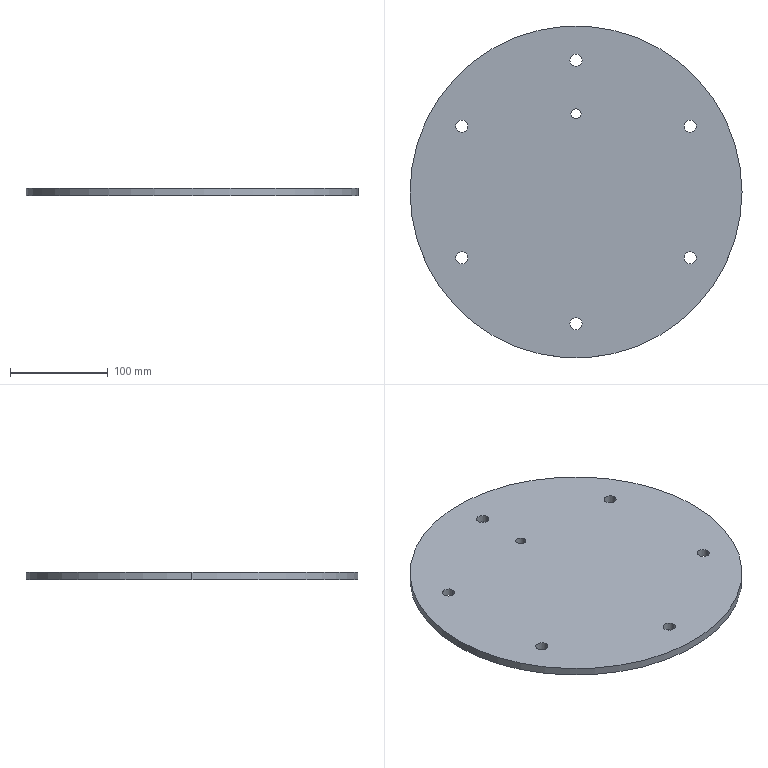Part | SolidWorks | features ICE 2, Extrusion 1 | 1 solid | 18 faces | box 340 x 340 x 8 mm | volume 719786 mm3 | cylinder 16 | plane 2 | commonest cylinder face diameters 12.5 x12 10.25 x2 340 x2
STEP:
#1=CARTESIAN_POINT('',(-5.125,80.,8.));
#2=VERTEX_POINT('',#1);
#3=CARTESIAN_POINT('',(5.125,80.,8.));
#4=VERTEX_POINT('',#3);
#5=CARTESIAN_POINT('',(0.,80.,8.));
#6=DIRECTION('',(0.,0.,1.));
#7=DIRECTION('',(1.,0.,0.));
#8=AXIS2_PLACEMENT_3D('',#5,#6,#7);
#9=CIRCLE('',#8,5.125);
#10=EDGE_CURVE('',#2,#4,#9,.T.);
#11=ORIENTED_EDGE('',*,*,#10,.T.);
#12=CARTESIAN_POINT('',(5.125,80.,0.));
#13=VERTEX_POINT('',#12);
#14=CARTESIAN_POINT('',(5.125,80.,10.));
#15=DIRECTION('',(0.,0.,-1.));
#16=VECTOR('',#15,1000.);
#17=LINE('',#14,#16);
#18=EDGE_CURVE('',#4,#13,#17,.T.);
#19=ORIENTED_EDGE('',*,*,#18,.T.);
#20=CARTESIAN_POINT('',(-5.125,80.,0.));
#21=VERTEX_POINT('',#20);
#22=CARTESIAN_POINT('',(0.,80.,0.));
#23=DIRECTION('',(0.,0.,-1.));
#24=DIRECTION('',(-1.,0.,0.));
#25=AXIS2_PLACEMENT_3D('',#22,#23,#24);
#26=CIRCLE('',#25,5.125);
#27=EDGE_CURVE('',#13,#21,#26,.T.);
#28=ORIENTED_EDGE('',*,*,#27,.T.);
#29=CARTESIAN_POINT('',(-5.125,80.,10.));
#30=DIRECTION('',(0.,0.,-1.));
#31=VECTOR('',#30,1000.);
#32=LINE('',#29,#31);
#33=EDGE_CURVE('',#2,#21,#32,.T.);
#34=ORIENTED_EDGE('',*,*,#33,.F.);
#35=EDGE_LOOP('',(#11,#19,#28,#34));
#36=FACE_OUTER_BOUND('',#35,.T.);
#37=CARTESIAN_POINT('',(0.,80.,10.));
#38=DIRECTION('',(0.,0.,-1.));
#39=DIRECTION('',(-1.,0.,0.));
#40=AXIS2_PLACEMENT_3D('',#37,#38,#39);
#41=CYLINDRICAL_SURFACE('',#40,5.125);
#42=ADVANCED_FACE('',(#36),#41,.F.);
#43=CARTESIAN_POINT('',(110.663,67.5,8.));
#44=VERTEX_POINT('',#43);
#45=CARTESIAN_POINT('',(123.163,67.5,8.));
#46=VERTEX_POINT('',#45);
#47=CARTESIAN_POINT('',(116.913,67.5,8.));
#48=DIRECTION('',(0.,0.,1.));
#49=DIRECTION('',(1.,0.,0.));
#50=AXIS2_PLACEMENT_3D('',#47,#48,#49);
#51=CIRCLE('',#50,6.25);
#52=EDGE_CURVE('',#44,#46,#51,.T.);
#53=ORIENTED_EDGE('',*,*,#52,.T.);
#54=CARTESIAN_POINT('',(123.163,67.5,0.));
#55=VERTEX_POINT('',#54);
#56=CARTESIAN_POINT('',(123.163,67.5,10.));
#57=DIRECTION('',(0.,0.,-1.));
#58=VECTOR('',#57,1000.);
#59=LINE('',#56,#58);
#60=EDGE_CURVE('',#46,#55,#59,.T.);
#61=ORIENTED_EDGE('',*,*,#60,.T.);
#62=CARTESIAN_POINT('',(110.663,67.5,0.));
#63=VERTEX_POINT('',#62);
#64=CARTESIAN_POINT('',(116.913,67.5,0.));
#65=DIRECTION('',(0.,0.,-1.));
#66=DIRECTION('',(-1.,0.,0.));
#67=AXIS2_PLACEMENT_3D('',#64,#65,#66);
#68=CIRCLE('',#67,6.25);
#69=EDGE_CURVE('',#55,#63,#68,.T.);
#70=ORIENTED_EDGE('',*,*,#69,.T.);
#71=CARTESIAN_POINT('',(110.663,67.5,10.));
#72=DIRECTION('',(0.,0.,-1.));
#73=VECTOR('',#72,1000.);
#74=LINE('',#71,#73);
#75=EDGE_CURVE('',#44,#63,#74,.T.);
#76=ORIENTED_EDGE('',*,*,#75,.F.);
#77=EDGE_LOOP('',(#53,#61,#70,#76));
#78=FACE_OUTER_BOUND('',#77,.T.);
#79=CARTESIAN_POINT('',(116.913,67.5,10.));
#80=DIRECTION('',(0.,0.,-1.));
#81=DIRECTION('',(-1.,0.,0.));
#82=AXIS2_PLACEMENT_3D('',#79,#80,#81);
#83=CYLINDRICAL_SURFACE('',#82,6.25);
#84=ADVANCED_FACE('',(#78),#83,.F.);
#85=CARTESIAN_POINT('',(110.663,-67.5,8.));
#86=VERTEX_POINT('',#85);
#87=CARTESIAN_POINT('',(123.163,-67.5,8.));
#88=VERTEX_POINT('',#87);
#89=CARTESIAN_POINT('',(116.913,-67.5,8.));
#90=DIRECTION('',(0.,0.,1.));
#91=DIRECTION('',(1.,0.,0.));
#92=AXIS2_PLACEMENT_3D('',#89,#90,#91);
#93=CIRCLE('',#92,6.25);
#94=EDGE_CURVE('',#86,#88,#93,.T.);
#95=ORIENTED_EDGE('',*,*,#94,.T.);
#96=CARTESIAN_POINT('',(123.163,-67.5,0.));
#97=VERTEX_POINT('',#96);
#98=CARTESIAN_POINT('',(123.163,-67.5,10.));
#99=DIRECTION('',(0.,0.,-1.));
#100=VECTOR('',#99,1000.);
#101=LINE('',#98,#100);
#102=EDGE_CURVE('',#88,#97,#101,.T.);
#103=ORIENTED_EDGE('',*,*,#102,.T.);
#104=CARTESIAN_POINT('',(110.663,-67.5,0.));
#105=VERTEX_POINT('',#104);
#106=CARTESIAN_POINT('',(116.913,-67.5,0.));
#107=DIRECTION('',(0.,0.,-1.));
#108=DIRECTION('',(-1.,0.,0.));
#109=AXIS2_PLACEMENT_3D('',#106,#107,#108);
#110=CIRCLE('',#109,6.25);
#111=EDGE_CURVE('',#97,#105,#110,.T.);
#112=ORIENTED_EDGE('',*,*,#111,.T.);
#113=CARTESIAN_POINT('',(110.663,-67.5,10.));
#114=DIRECTION('',(0.,0.,-1.));
#115=VECTOR('',#114,1000.);
#116=LINE('',#113,#115);
#117=EDGE_CURVE('',#86,#105,#116,.T.);
#118=ORIENTED_EDGE('',*,*,#117,.F.);
#119=EDGE_LOOP('',(#95,#103,#112,#118));
#120=FACE_OUTER_BOUND('',#119,.T.);
#121=CARTESIAN_POINT('',(116.913,-67.5,10.));
#122=DIRECTION('',(0.,0.,-1.));
#123=DIRECTION('',(-1.,0.,0.));
#124=AXIS2_PLACEMENT_3D('',#121,#122,#123);
#125=CYLINDRICAL_SURFACE('',#124,6.25);
#126=ADVANCED_FACE('',(#120),#125,.F.);
#127=CARTESIAN_POINT('',(-6.25,-135.,8.));
#128=VERTEX_POINT('',#127);
#129=CARTESIAN_POINT('',(6.25,-135.,8.));
#130=VERTEX_POINT('',#129);
#131=CARTESIAN_POINT('',(0.,-135.,8.));
#132=DIRECTION('',(0.,0.,1.));
#133=DIRECTION('',(1.,0.,0.));
#134=AXIS2_PLACEMENT_3D('',#131,#132,#133);
#135=CIRCLE('',#134,6.25);
#136=EDGE_CURVE('',#128,#130,#135,.T.);
#137=ORIENTED_EDGE('',*,*,#136,.T.);
#138=CARTESIAN_POINT('',(6.25,-135.,0.));
#139=VERTEX_POINT('',#138);
#140=CARTESIAN_POINT('',(6.25,-135.,10.));
#141=DIRECTION('',(0.,0.,-1.));
#142=VECTOR('',#141,1000.);
#143=LINE('',#140,#142);
#144=EDGE_CURVE('',#130,#139,#143,.T.);
#145=ORIENTED_EDGE('',*,*,#144,.T.);
#146=CARTESIAN_POINT('',(-6.25,-135.,0.));
#147=VERTEX_POINT('',#146);
#148=CARTESIAN_POINT('',(0.,-135.,0.));
#149=DIRECTION('',(0.,0.,-1.));
#150=DIRECTION('',(-1.,0.,0.));
#151=AXIS2_PLACEMENT_3D('',#148,#149,#150);
#152=CIRCLE('',#151,6.25);
#153=EDGE_CURVE('',#139,#147,#152,.T.);
#154=ORIENTED_EDGE('',*,*,#153,.T.);
#155=CARTESIAN_POINT('',(-6.25,-135.,10.));
#156=DIRECTION('',(0.,0.,-1.));
#157=VECTOR('',#156,1000.);
#158=LINE('',#155,#157);
#159=EDGE_CURVE('',#128,#147,#158,.T.);
#160=ORIENTED_EDGE('',*,*,#159,.F.);
#161=EDGE_LOOP('',(#137,#145,#154,#160));
#162=FACE_OUTER_BOUND('',#161,.T.);
#163=CARTESIAN_POINT('',(0.,-135.,10.));
#164=DIRECTION('',(0.,0.,-1.));
#165=DIRECTION('',(-1.,0.,0.));
#166=AXIS2_PLACEMENT_3D('',#163,#164,#165);
#167=CYLINDRICAL_SURFACE('',#166,6.25);
#168=ADVANCED_FACE('',(#162),#167,.F.);
#169=CARTESIAN_POINT('',(-123.163,-67.5,8.));
#170=VERTEX_POINT('',#169);
#171=CARTESIAN_POINT('',(-110.663,-67.5,8.));
#172=VERTEX_POINT('',#171);
#173=CARTESIAN_POINT('',(-116.913,-67.5,8.));
#174=DIRECTION('',(0.,0.,1.));
#175=DIRECTION('',(1.,0.,0.));
#176=AXIS2_PLACEMENT_3D('',#173,#174,#175);
#177=CIRCLE('',#176,6.25);
#178=EDGE_CURVE('',#170,#172,#177,.T.);
#179=ORIENTED_EDGE('',*,*,#178,.T.);
#180=CARTESIAN_POINT('',(-110.663,-67.5,0.));
#181=VERTEX_POINT('',#180);
#182=CARTESIAN_POINT('',(-110.663,-67.5,10.));
#183=DIRECTION('',(0.,0.,-1.));
#184=VECTOR('',#183,1000.);
#185=LINE('',#182,#184);
#186=EDGE_CURVE('',#172,#181,#185,.T.);
#187=ORIENTED_EDGE('',*,*,#186,.T.);
#188=CARTESIAN_POINT('',(-123.163,-67.5,0.));
#189=VERTEX_POINT('',#188);
#190=CARTESIAN_POINT('',(-116.913,-67.5,0.));
#191=DIRECTION('',(0.,0.,-1.));
#192=DIRECTION('',(-1.,0.,0.));
#193=AXIS2_PLACEMENT_3D('',#190,#191,#192);
#194=CIRCLE('',#193,6.25);
#195=EDGE_CURVE('',#181,#189,#194,.T.);
#196=ORIENTED_EDGE('',*,*,#195,.T.);
#197=CARTESIAN_POINT('',(-123.163,-67.5,10.));
#198=DIRECTION('',(0.,0.,-1.));
#199=VECTOR('',#198,1000.);
#200=LINE('',#197,#199);
#201=EDGE_CURVE('',#170,#189,#200,.T.);
#202=ORIENTED_EDGE('',*,*,#201,.F.);
#203=EDGE_LOOP('',(#179,#187,#196,#202));
#204=FACE_OUTER_BOUND('',#203,.T.);
#205=CARTESIAN_POINT('',(-116.913,-67.5,10.));
#206=DIRECTION('',(0.,0.,-1.));
#207=DIRECTION('',(-1.,0.,0.));
#208=AXIS2_PLACEMENT_3D('',#205,#206,#207);
#209=CYLINDRICAL_SURFACE('',#208,6.25);
#210=ADVANCED_FACE('',(#204),#209,.F.);
#211=CARTESIAN_POINT('',(-123.163,67.5,8.));
#212=VERTEX_POINT('',#211);
#213=CARTESIAN_POINT('',(-110.663,67.5,8.));
#214=VERTEX_POINT('',#213);
#215=CARTESIAN_POINT('',(-116.913,67.5,8.));
#216=DIRECTION('',(0.,0.,1.));
#217=DIRECTION('',(1.,0.,0.));
#218=AXIS2_PLACEMENT_3D('',#215,#216,#217);
#219=CIRCLE('',#218,6.25);
#220=EDGE_CURVE('',#212,#214,#219,.T.);
#221=ORIENTED_EDGE('',*,*,#220,.T.);
#222=CARTESIAN_POINT('',(-110.663,67.5,0.));
#223=VERTEX_POINT('',#222);
#224=CARTESIAN_POINT('',(-110.663,67.5,10.));
#225=DIRECTION('',(0.,0.,-1.));
#226=VECTOR('',#225,1000.);
#227=LINE('',#224,#226);
#228=EDGE_CURVE('',#214,#223,#227,.T.);
#229=ORIENTED_EDGE('',*,*,#228,.T.);
#230=CARTESIAN_POINT('',(-123.163,67.5,0.));
#231=VERTEX_POINT('',#230);
#232=CARTESIAN_POINT('',(-116.913,67.5,0.));
#233=DIRECTION('',(0.,0.,-1.));
#234=DIRECTION('',(-1.,0.,0.));
#235=AXIS2_PLACEMENT_3D('',#232,#233,#234);
#236=CIRCLE('',#235,6.25);
#237=EDGE_CURVE('',#223,#231,#236,.T.);
#238=ORIENTED_EDGE('',*,*,#237,.T.);
#239=CARTESIAN_POINT('',(-123.163,67.5,10.));
#240=DIRECTION('',(0.,0.,-1.));
#241=VECTOR('',#240,1000.);
#242=LINE('',#239,#241);
#243=EDGE_CURVE('',#212,#231,#242,.T.);
#244=ORIENTED_EDGE('',*,*,#243,.F.);
#245=EDGE_LOOP('',(#221,#229,#238,#244));
#246=FACE_OUTER_BOUND('',#245,.T.);
#247=CARTESIAN_POINT('',(-116.913,67.5,10.));
#248=DIRECTION('',(0.,0.,-1.));
#249=DIRECTION('',(-1.,0.,0.));
#250=AXIS2_PLACEMENT_3D('',#247,#248,#249);
#251=CYLINDRICAL_SURFACE('',#250,6.25);
#252=ADVANCED_FACE('',(#246),#251,.F.);
#253=CARTESIAN_POINT('',(-6.25,135.,8.));
#254=VERTEX_POINT('',#253);
#255=CARTESIAN_POINT('',(6.25,135.,8.));
#256=VERTEX_POINT('',#255);
#257=CARTESIAN_POINT('',(0.,135.,8.));
#258=DIRECTION('',(0.,0.,1.));
#259=DIRECTION('',(1.,0.,0.));
#260=AXIS2_PLACEMENT_3D('',#257,#258,#259);
#261=CIRCLE('',#260,6.25);
#262=EDGE_CURVE('',#254,#256,#261,.T.);
#263=ORIENTED_EDGE('',*,*,#262,.T.);
#264=CARTESIAN_POINT('',(6.25,135.,0.));
#265=VERTEX_POINT('',#264);
#266=CARTESIAN_POINT('',(6.25,135.,10.));
#267=DIRECTION('',(0.,0.,-1.));
#268=VECTOR('',#267,1000.);
#269=LINE('',#266,#268);
#270=EDGE_CURVE('',#256,#265,#269,.T.);
#271=ORIENTED_EDGE('',*,*,#270,.T.);
#272=CARTESIAN_POINT('',(-6.25,135.,0.));
#273=VERTEX_POINT('',#272);
#274=CARTESIAN_POINT('',(0.,135.,0.));
#275=DIRECTION('',(0.,0.,-1.));
#276=DIRECTION('',(-1.,0.,0.));
#277=AXIS2_PLACEMENT_3D('',#274,#275,#276);
#278=CIRCLE('',#277,6.25);
#279=EDGE_CURVE('',#265,#273,#278,.T.);
#280=ORIENTED_EDGE('',*,*,#279,.T.);
#281=CARTESIAN_POINT('',(-6.25,135.,10.));
#282=DIRECTION('',(0.,0.,-1.));
#283=VECTOR('',#282,1000.);
#284=LINE('',#281,#283);
#285=EDGE_CURVE('',#254,#273,#284,.T.);
#286=ORIENTED_EDGE('',*,*,#285,.F.);
#287=EDGE_LOOP('',(#263,#271,#280,#286));
#288=FACE_OUTER_BOUND('',#287,.T.);
#289=CARTESIAN_POINT('',(0.,135.,10.));
#290=DIRECTION('',(0.,0.,-1.));
#291=DIRECTION('',(-1.,0.,0.));
#292=AXIS2_PLACEMENT_3D('',#289,#290,#291);
#293=CYLINDRICAL_SURFACE('',#292,6.25);
#294=ADVANCED_FACE('',(#288),#293,.F.);
#295=CARTESIAN_POINT('',(170.,0.,8.));
#296=VERTEX_POINT('',#295);
#297=CARTESIAN_POINT('',(-170.,0.,8.));
#298=VERTEX_POINT('',#297);
#299=CARTESIAN_POINT('',(0.,0.,8.));
#300=DIRECTION('',(0.,0.,1.));
#301=DIRECTION('',(1.,0.,0.));
#302=AXIS2_PLACEMENT_3D('',#299,#300,#301);
#303=CIRCLE('',#302,170.);
#304=EDGE_CURVE('',#296,#298,#303,.T.);
#305=ORIENTED_EDGE('',*,*,#304,.F.);
#306=CARTESIAN_POINT('',(170.,0.,0.));
#307=VERTEX_POINT('',#306);
#308=CARTESIAN_POINT('',(170.,0.,8.));
#309=DIRECTION('',(0.,0.,-1.));
#310=VECTOR('',#309,1000.);
#311=LINE('',#308,#310);
#312=EDGE_CURVE('',#296,#307,#311,.T.);
#313=ORIENTED_EDGE('',*,*,#312,.T.);
#314=CARTESIAN_POINT('',(-170.,0.,0.));
#315=VERTEX_POINT('',#314);
#316=CARTESIAN_POINT('',(0.,0.,0.));
#317=DIRECTION('',(0.,0.,1.));
#318=DIRECTION('',(1.,0.,0.));
#319=AXIS2_PLACEMENT_3D('',#316,#317,#318);
#320=CIRCLE('',#319,170.);
#321=EDGE_CURVE('',#307,#315,#320,.T.);
#322=ORIENTED_EDGE('',*,*,#321,.T.);
#323=CARTESIAN_POINT('',(-170.,0.,8.));
#324=DIRECTION('',(0.,0.,-1.));
#325=VECTOR('',#324,1000.);
#326=LINE('',#323,#325);
#327=EDGE_CURVE('',#298,#315,#326,.T.);
#328=ORIENTED_EDGE('',*,*,#327,.F.);
#329=EDGE_LOOP('',(#305,#313,#322,#328));
#330=FACE_OUTER_BOUND('',#329,.T.);
#331=CARTESIAN_POINT('',(0.,0.,8.));
#332=DIRECTION('',(0.,0.,-1.));
#333=DIRECTION('',(-1.,0.,0.));
#334=AXIS2_PLACEMENT_3D('',#331,#332,#333);
#335=CYLINDRICAL_SURFACE('',#334,170.);
#336=ADVANCED_FACE('',(#330),#335,.T.);
#337=ORIENTED_EDGE('',*,*,#312,.F.);
#338=CARTESIAN_POINT('',(0.,0.,8.));
#339=DIRECTION('',(0.,0.,1.));
#340=DIRECTION('',(1.,0.,0.));
#341=AXIS2_PLACEMENT_3D('',#338,#339,#340);
#342=CIRCLE('',#341,170.);
#343=EDGE_CURVE('',#298,#296,#342,.T.);
#344=ORIENTED_EDGE('',*,*,#343,.F.);
#345=ORIENTED_EDGE('',*,*,#327,.T.);
#346=CARTESIAN_POINT('',(0.,0.,0.));
#347=DIRECTION('',(0.,0.,1.));
#348=DIRECTION('',(1.,0.,0.));
#349=AXIS2_PLACEMENT_3D('',#346,#347,#348);
#350=CIRCLE('',#349,170.);
#351=EDGE_CURVE('',#315,#307,#350,.T.);
#352=ORIENTED_EDGE('',*,*,#351,.T.);
#353=EDGE_LOOP('',(#337,#344,#345,#352));
#354=FACE_OUTER_BOUND('',#353,.T.);
#355=CARTESIAN_POINT('',(0.,0.,8.));
#356=DIRECTION('',(0.,0.,-1.));
#357=DIRECTION('',(-1.,0.,0.));
#358=AXIS2_PLACEMENT_3D('',#355,#356,#357);
#359=CYLINDRICAL_SURFACE('',#358,170.);
#360=ADVANCED_FACE('',(#354),#359,.T.);
#361=ORIENTED_EDGE('',*,*,#10,.F.);
#362=CARTESIAN_POINT('',(0.,80.,8.));
#363=DIRECTION('',(0.,0.,1.));
#364=DIRECTION('',(1.,0.,0.));
#365=AXIS2_PLACEMENT_3D('',#362,#363,#364);
#366=CIRCLE('',#365,5.125);
#367=EDGE_CURVE('',#4,#2,#366,.T.);
#368=ORIENTED_EDGE('',*,*,#367,.F.);
#369=EDGE_LOOP('',(#361,#368));
#370=FACE_BOUND('',#369,.T.);
#371=ORIENTED_EDGE('',*,*,#52,.F.);
#372=CARTESIAN_POINT('',(116.913,67.5,8.));
#373=DIRECTION('',(0.,0.,1.));
#374=DIRECTION('',(1.,0.,0.));
#375=AXIS2_PLACEMENT_3D('',#372,#373,#374);
#376=CIRCLE('',#375,6.25);
#377=EDGE_CURVE('',#46,#44,#376,.T.);
#378=ORIENTED_EDGE('',*,*,#377,.F.);
#379=EDGE_LOOP('',(#371,#378));
#380=FACE_BOUND('',#379,.T.);
#381=ORIENTED_EDGE('',*,*,#94,.F.);
#382=CARTESIAN_POINT('',(116.913,-67.5,8.));
#383=DIRECTION('',(0.,0.,1.));
#384=DIRECTION('',(1.,0.,0.));
#385=AXIS2_PLACEMENT_3D('',#382,#383,#384);
#386=CIRCLE('',#385,6.25);
#387=EDGE_CURVE('',#88,#86,#386,.T.);
#388=ORIENTED_EDGE('',*,*,#387,.F.);
#389=EDGE_LOOP('',(#381,#388));
#390=FACE_BOUND('',#389,.T.);
#391=ORIENTED_EDGE('',*,*,#136,.F.);
#392=CARTESIAN_POINT('',(0.,-135.,8.));
#393=DIRECTION('',(0.,0.,1.));
#394=DIRECTION('',(1.,0.,0.));
#395=AXIS2_PLACEMENT_3D('',#392,#393,#394);
#396=CIRCLE('',#395,6.25);
#397=EDGE_CURVE('',#130,#128,#396,.T.);
#398=ORIENTED_EDGE('',*,*,#397,.F.);
#399=EDGE_LOOP('',(#391,#398));
#400=FACE_BOUND('',#399,.T.);
#401=ORIENTED_EDGE('',*,*,#178,.F.);
#402=CARTESIAN_POINT('',(-116.913,-67.5,8.));
#403=DIRECTION('',(0.,0.,1.));
#404=DIRECTION('',(1.,0.,0.));
#405=AXIS2_PLACEMENT_3D('',#402,#403,#404);
#406=CIRCLE('',#405,6.25);
#407=EDGE_CURVE('',#172,#170,#406,.T.);
#408=ORIENTED_EDGE('',*,*,#407,.F.);
#409=EDGE_LOOP('',(#401,#408));
#410=FACE_BOUND('',#409,.T.);
#411=ORIENTED_EDGE('',*,*,#220,.F.);
#412=CARTESIAN_POINT('',(-116.913,67.5,8.));
#413=DIRECTION('',(0.,0.,1.));
#414=DIRECTION('',(1.,0.,0.));
#415=AXIS2_PLACEMENT_3D('',#412,#413,#414);
#416=CIRCLE('',#415,6.25);
#417=EDGE_CURVE('',#214,#212,#416,.T.);
#418=ORIENTED_EDGE('',*,*,#417,.F.);
#419=EDGE_LOOP('',(#411,#418));
#420=FACE_BOUND('',#419,.T.);
#421=ORIENTED_EDGE('',*,*,#262,.F.);
#422=CARTESIAN_POINT('',(0.,135.,8.));
#423=DIRECTION('',(0.,0.,1.));
#424=DIRECTION('',(1.,0.,0.));
#425=AXIS2_PLACEMENT_3D('',#422,#423,#424);
#426=CIRCLE('',#425,6.25);
#427=EDGE_CURVE('',#256,#254,#426,.T.);
#428=ORIENTED_EDGE('',*,*,#427,.F.);
#429=EDGE_LOOP('',(#421,#428));
#430=FACE_BOUND('',#429,.T.);
#431=ORIENTED_EDGE('',*,*,#343,.T.);
#432=ORIENTED_EDGE('',*,*,#304,.T.);
#433=EDGE_LOOP('',(#431,#432));
#434=FACE_OUTER_BOUND('',#433,.T.);
#435=CARTESIAN_POINT('',(0.,0.,8.));
#436=DIRECTION('',(0.,0.,1.));
#437=DIRECTION('',(1.,0.,0.));
#438=AXIS2_PLACEMENT_3D('',#435,#436,#437);
#439=PLANE('',#438);
#440=ADVANCED_FACE('',(#370,#380,#390,#400,#410,#420,#430,#434),#439,.T.);
#441=CARTESIAN_POINT('',(0.,80.,0.));
#442=DIRECTION('',(0.,0.,-1.));
#443=DIRECTION('',(-1.,0.,0.));
#444=AXIS2_PLACEMENT_3D('',#441,#442,#443);
#445=CIRCLE('',#444,5.125);
#446=EDGE_CURVE('',#21,#13,#445,.T.);
#447=ORIENTED_EDGE('',*,*,#446,.F.);
#448=ORIENTED_EDGE('',*,*,#27,.F.);
#449=EDGE_LOOP('',(#447,#448));
#450=FACE_BOUND('',#449,.T.);
#451=CARTESIAN_POINT('',(116.913,67.5,0.));
#452=DIRECTION('',(0.,0.,-1.));
#453=DIRECTION('',(-1.,0.,0.));
#454=AXIS2_PLACEMENT_3D('',#451,#452,#453);
#455=CIRCLE('',#454,6.25);
#456=EDGE_CURVE('',#63,#55,#455,.T.);
#457=ORIENTED_EDGE('',*,*,#456,.F.);
#458=ORIENTED_EDGE('',*,*,#69,.F.);
#459=EDGE_LOOP('',(#457,#458));
#460=FACE_BOUND('',#459,.T.);
#461=CARTESIAN_POINT('',(116.913,-67.5,0.));
#462=DIRECTION('',(0.,0.,-1.));
#463=DIRECTION('',(-1.,0.,0.));
#464=AXIS2_PLACEMENT_3D('',#461,#462,#463);
#465=CIRCLE('',#464,6.25);
#466=EDGE_CURVE('',#105,#97,#465,.T.);
#467=ORIENTED_EDGE('',*,*,#466,.F.);
#468=ORIENTED_EDGE('',*,*,#111,.F.);
#469=EDGE_LOOP('',(#467,#468));
#470=FACE_BOUND('',#469,.T.);
#471=CARTESIAN_POINT('',(0.,-135.,0.));
#472=DIRECTION('',(0.,0.,-1.));
#473=DIRECTION('',(-1.,0.,0.));
#474=AXIS2_PLACEMENT_3D('',#471,#472,#473);
#475=CIRCLE('',#474,6.25);
#476=EDGE_CURVE('',#147,#139,#475,.T.);
#477=ORIENTED_EDGE('',*,*,#476,.F.);
#478=ORIENTED_EDGE('',*,*,#153,.F.);
#479=EDGE_LOOP('',(#477,#478));
#480=FACE_BOUND('',#479,.T.);
#481=CARTESIAN_POINT('',(-116.913,-67.5,0.));
#482=DIRECTION('',(0.,0.,-1.));
#483=DIRECTION('',(-1.,0.,0.));
#484=AXIS2_PLACEMENT_3D('',#481,#482,#483);
#485=CIRCLE('',#484,6.25);
#486=EDGE_CURVE('',#189,#181,#485,.T.);
#487=ORIENTED_EDGE('',*,*,#486,.F.);
#488=ORIENTED_EDGE('',*,*,#195,.F.);
#489=EDGE_LOOP('',(#487,#488));
#490=FACE_BOUND('',#489,.T.);
#491=CARTESIAN_POINT('',(-116.913,67.5,0.));
#492=DIRECTION('',(0.,0.,-1.));
#493=DIRECTION('',(-1.,0.,0.));
#494=AXIS2_PLACEMENT_3D('',#491,#492,#493);
#495=CIRCLE('',#494,6.25);
#496=EDGE_CURVE('',#231,#223,#495,.T.);
#497=ORIENTED_EDGE('',*,*,#496,.F.);
#498=ORIENTED_EDGE('',*,*,#237,.F.);
#499=EDGE_LOOP('',(#497,#498));
#500=FACE_BOUND('',#499,.T.);
#501=CARTESIAN_POINT('',(0.,135.,0.));
#502=DIRECTION('',(0.,0.,-1.));
#503=DIRECTION('',(-1.,0.,0.));
#504=AXIS2_PLACEMENT_3D('',#501,#502,#503);
#505=CIRCLE('',#504,6.25);
#506=EDGE_CURVE('',#273,#265,#505,.T.);
#507=ORIENTED_EDGE('',*,*,#506,.F.);
#508=ORIENTED_EDGE('',*,*,#279,.F.);
#509=EDGE_LOOP('',(#507,#508));
#510=FACE_BOUND('',#509,.T.);
#511=ORIENTED_EDGE('',*,*,#351,.F.);
#512=ORIENTED_EDGE('',*,*,#321,.F.);
#513=EDGE_LOOP('',(#511,#512));
#514=FACE_OUTER_BOUND('',#513,.T.);
#515=CARTESIAN_POINT('',(0.,0.,0.));
#516=DIRECTION('',(0.,0.,1.));
#517=DIRECTION('',(1.,0.,0.));
#518=AXIS2_PLACEMENT_3D('',#515,#516,#517);
#519=PLANE('',#518);
#520=ADVANCED_FACE('',(#450,#460,#470,#480,#490,#500,#510,#514),#519,.F.);
#521=ORIENTED_EDGE('',*,*,#270,.F.);
#522=ORIENTED_EDGE('',*,*,#427,.T.);
#523=ORIENTED_EDGE('',*,*,#285,.T.);
#524=ORIENTED_EDGE('',*,*,#506,.T.);
#525=EDGE_LOOP('',(#521,#522,#523,#524));
#526=FACE_OUTER_BOUND('',#525,.T.);
#527=CARTESIAN_POINT('',(0.,135.,10.));
#528=DIRECTION('',(0.,0.,-1.));
#529=DIRECTION('',(-1.,0.,0.));
#530=AXIS2_PLACEMENT_3D('',#527,#528,#529);
#531=CYLINDRICAL_SURFACE('',#530,6.25);
#532=ADVANCED_FACE('',(#526),#531,.F.);
#533=ORIENTED_EDGE('',*,*,#228,.F.);
#534=ORIENTED_EDGE('',*,*,#417,.T.);
#535=ORIENTED_EDGE('',*,*,#243,.T.);
#536=ORIENTED_EDGE('',*,*,#496,.T.);
#537=EDGE_LOOP('',(#533,#534,#535,#536));
#538=FACE_OUTER_BOUND('',#537,.T.);
#539=CARTESIAN_POINT('',(-116.913,67.5,10.));
#540=DIRECTION('',(0.,0.,-1.));
#541=DIRECTION('',(-1.,0.,0.));
#542=AXIS2_PLACEMENT_3D('',#539,#540,#541);
#543=CYLINDRICAL_SURFACE('',#542,6.25);
#544=ADVANCED_FACE('',(#538),#543,.F.);
#545=ORIENTED_EDGE('',*,*,#186,.F.);
#546=ORIENTED_EDGE('',*,*,#407,.T.);
#547=ORIENTED_EDGE('',*,*,#201,.T.);
#548=ORIENTED_EDGE('',*,*,#486,.T.);
#549=EDGE_LOOP('',(#545,#546,#547,#548));
#550=FACE_OUTER_BOUND('',#549,.T.);
#551=CARTESIAN_POINT('',(-116.913,-67.5,10.));
#552=DIRECTION('',(0.,0.,-1.));
#553=DIRECTION('',(-1.,0.,0.));
#554=AXIS2_PLACEMENT_3D('',#551,#552,#553);
#555=CYLINDRICAL_SURFACE('',#554,6.25);
#556=ADVANCED_FACE('',(#550),#555,.F.);
#557=ORIENTED_EDGE('',*,*,#144,.F.);
#558=ORIENTED_EDGE('',*,*,#397,.T.);
#559=ORIENTED_EDGE('',*,*,#159,.T.);
#560=ORIENTED_EDGE('',*,*,#476,.T.);
#561=EDGE_LOOP('',(#557,#558,#559,#560));
#562=FACE_OUTER_BOUND('',#561,.T.);
#563=CARTESIAN_POINT('',(0.,-135.,10.));
#564=DIRECTION('',(0.,0.,-1.));
#565=DIRECTION('',(-1.,0.,0.));
#566=AXIS2_PLACEMENT_3D('',#563,#564,#565);
#567=CYLINDRICAL_SURFACE('',#566,6.25);
#568=ADVANCED_FACE('',(#562),#567,.F.);
#569=ORIENTED_EDGE('',*,*,#102,.F.);
#570=ORIENTED_EDGE('',*,*,#387,.T.);
#571=ORIENTED_EDGE('',*,*,#117,.T.);
#572=ORIENTED_EDGE('',*,*,#466,.T.);
#573=EDGE_LOOP('',(#569,#570,#571,#572));
#574=FACE_OUTER_BOUND('',#573,.T.);
#575=CARTESIAN_POINT('',(116.913,-67.5,10.));
#576=DIRECTION('',(0.,0.,-1.));
#577=DIRECTION('',(-1.,0.,0.));
#578=AXIS2_PLACEMENT_3D('',#575,#576,#577);
#579=CYLINDRICAL_SURFACE('',#578,6.25);
#580=ADVANCED_FACE('',(#574),#579,.F.);
#581=ORIENTED_EDGE('',*,*,#60,.F.);
#582=ORIENTED_EDGE('',*,*,#377,.T.);
#583=ORIENTED_EDGE('',*,*,#75,.T.);
#584=ORIENTED_EDGE('',*,*,#456,.T.);
#585=EDGE_LOOP('',(#581,#582,#583,#584));
#586=FACE_OUTER_BOUND('',#585,.T.);
#587=CARTESIAN_POINT('',(116.913,67.5,10.));
#588=DIRECTION('',(0.,0.,-1.));
#589=DIRECTION('',(-1.,0.,0.));
#590=AXIS2_PLACEMENT_3D('',#587,#588,#589);
#591=CYLINDRICAL_SURFACE('',#590,6.25);
#592=ADVANCED_FACE('',(#586),#591,.F.);
#593=ORIENTED_EDGE('',*,*,#18,.F.);
#594=ORIENTED_EDGE('',*,*,#367,.T.);
#595=ORIENTED_EDGE('',*,*,#33,.T.);
#596=ORIENTED_EDGE('',*,*,#446,.T.);
#597=EDGE_LOOP('',(#593,#594,#595,#596));
#598=FACE_OUTER_BOUND('',#597,.T.);
#599=CARTESIAN_POINT('',(0.,80.,10.));
#600=DIRECTION('',(0.,0.,-1.));
#601=DIRECTION('',(-1.,0.,0.));
#602=AXIS2_PLACEMENT_3D('',#599,#600,#601);
#603=CYLINDRICAL_SURFACE('',#602,5.125);
#604=ADVANCED_FACE('',(#598),#603,.F.);
#605=CLOSED_SHELL('',(#42,#84,#126,#168,#210,#252,#294,#336,#360,#440,#520,#532,#544,#556,#568,#580,#592,#604));
#606=MANIFOLD_SOLID_BREP('',#605);
#607=CARTESIAN_POINT('',(0.,0.,0.));
#608=DIRECTION('',(0.,0.,1.));
#609=DIRECTION('',(1.,0.,0.));
#610=AXIS2_PLACEMENT_3D('',#607,#608,#609);
#611=(LENGTH_UNIT()NAMED_UNIT(*)SI_UNIT(.MILLI.,.METRE.));
#612=UNCERTAINTY_MEASURE_WITH_UNIT(LENGTH_MEASURE(0.00001),#611,'','');
#613=(NAMED_UNIT(*)PLANE_ANGLE_UNIT()SI_UNIT($,.RADIAN.));
#614=(NAMED_UNIT(*)SI_UNIT($,.STERADIAN.)SOLID_ANGLE_UNIT());
#615=(GEOMETRIC_REPRESENTATION_CONTEXT(3)GLOBAL_UNCERTAINTY_ASSIGNED_CONTEXT((#612))GLOBAL_UNIT_ASSIGNED_CONTEXT((#611,#613,#614))REPRESENTATION_CONTEXT('',''));
#616=ADVANCED_BREP_SHAPE_REPRESENTATION('',(#606,#610),#615);